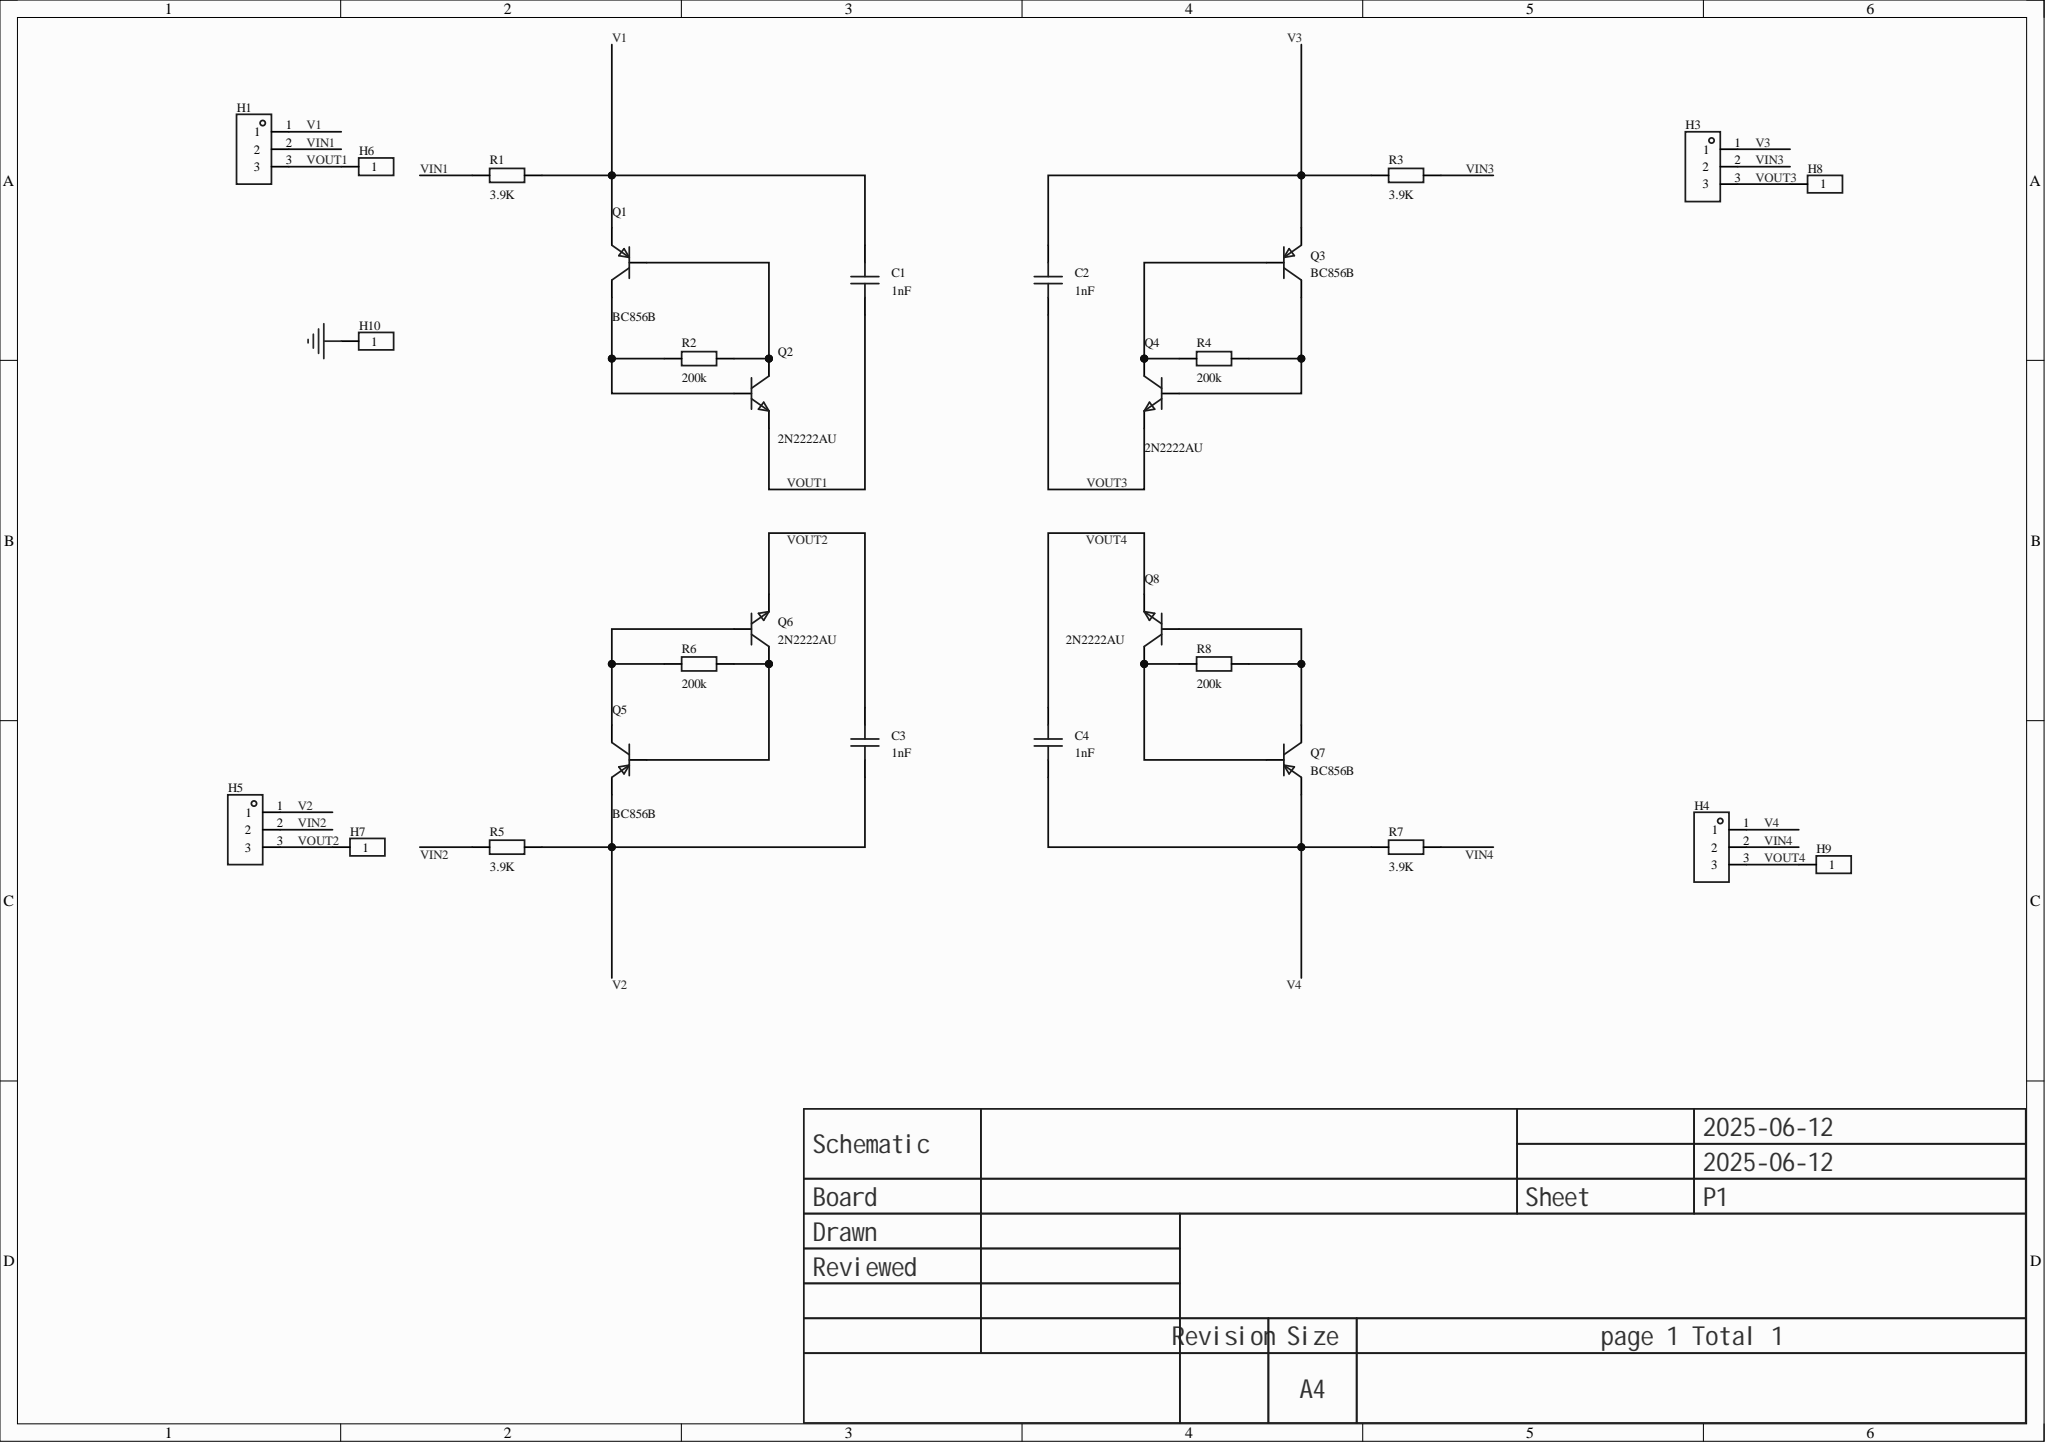Circuit board | Altium Designer | 29 parts | 20 nets
Bill of materials:
Comment,Description,Designator,Footprint,LibRef,Quantity
"1nF","","C1, C2, C3, C4","C0402","CAP_0402","4"
"","","H1, H3, H4, H5","HDR-TH_2P-P2.54-V-M-1","HDR-M_2.54_1x3P","4"
"","","H6, H7, H8, H9, H10","HDR-TH_1P-V-M_XKB_X4611WV-01I-C28D40","HDR-M_2.54_1x1P","5"
"BC856B","Transistor type: PNP; collector current (Ic): 100mA; collector-emitter breakdown voltage (Vceo): 65V; power dissipation (Pd): 200mW; DC current gain (hFE): 220@2mA,5V;","Q1, Q3, Q5, Q7","SOT-23-3_L2.9-W1.6-P1.90-LS2.8-BR","BC856B_C181144","4"
"2N2222AU","","Q2, Q4, Q6, Q8","SOT-89-3_L4.5-W2.4-P1.50-LS4.0-BR","2N2222AU","4"
"3.9K","","R1, R3, R5, R7","R0402","Res_0402","4"
"200k","","R2, R4, R6, R8","R0402","Res_0402","4"
Netlist (Protel format):
[
C1
C0402
1nF



]
[
C2
C0402
1nF



]
[
C3
C0402
1nF



]
[
C4
C0402
1nF



]
[
H1
HDR-TH_2P-P2.54-V-M-1




]
[
H3
HDR-TH_2P-P2.54-V-M-1




]
[
H4
HDR-TH_2P-P2.54-V-M-1




]
[
H5
HDR-TH_2P-P2.54-V-M-1




]
[
H6
HDR-TH_1P-V-M_XKB_X4611WV-01I-C28D40




]
[
H7
HDR-TH_1P-V-M_XKB_X4611WV-01I-C28D40




]
[
H8
HDR-TH_1P-V-M_XKB_X4611WV-01I-C28D40




]
[
H9
HDR-TH_1P-V-M_XKB_X4611WV-01I-C28D40




]
[
H10
HDR-TH_1P-V-M_XKB_X4611WV-01I-C28D40




]
[
Q1
SOT-23-3_L2.9-W1.6-P1.90-LS2.8-BR
BC856B



]
[
Q2
SOT-89-3_L4.5-W2.4-P1.50-LS4.0-BR
2N2222AU



]
[
Q3
SOT-23-3_L2.9-W1.6-P1.90-LS2.8-BR
BC856B



]
[
Q4
SOT-89-3_L4.5-W2.4-P1.50-LS4.0-BR
2N2222AU



]
[
Q5
SOT-23-3_L2.9-W1.6-P1.90-LS2.8-BR
BC856B



]
[
Q6
SOT-89-3_L4.5-W2.4-P1.50-LS4.0-BR
2N2222AU



]
[
Q7
SOT-23-3_L2.9-W1.6-P1.90-LS2.8-BR
BC856B



]
[
Q8
SOT-89-3_L4.5-W2.4-P1.50-LS4.0-BR
2N2222AU



]
[
R1
R0402
3.9K



]
[
R2
R0402
200k



]
[
R3
R0402
3.9K



]
[
R4
R0402
200k



]
[
R5
R0402
3.9K



]
[
R6
R0402
200k



]
[
R7
R0402
3.9K



]
[
R8
R0402
200k



]
(
VOUT4
C4-1
H4-3
H9-1
Q8-2
)
(
VOUT3
C2-1
H3-3
H8-1
Q4-2
)
(
VOUT2
C3-1
H5-3
H7-1
Q6-2
)
(
VOUT1
C1-1
H1-3
H6-1
Q2-2
)
(
VIN4
H4-2
R7-1
)
(
VIN3
H3-2
R3-1
)
(
VIN2
H5-2
R5-1
)
(
VIN1
H1-2
R1-1
)
(
V4
C4-2
H4-1
Q7-2
R7-2
)
(
V3
C2-2
H3-1
Q3-2
R3-2
)
(
V2
C3-2
H5-1
Q5-2
R5-2
)
(
V1
C1-2
H1-1
Q1-2
R1-2
)
(
NetQ7_3
Q7-3
Q8-1
R8-1
)
(
NetQ7_1
Q7-1
Q8-3
R8-2
)
(
NetQ5_3
Q5-3
Q6-1
R6-1
)
(
NetQ5_1
Q5-1
Q6-3
R6-2
)
(
NetQ3_3
Q3-3
Q4-1
R4-1
)
(
NetQ3_1
Q3-1
Q4-3
R4-2
)
(
NetQ1_3
Q1-3
Q2-1
R2-1
)
(
NetQ1_1
Q1-1
Q2-3
R2-2
)